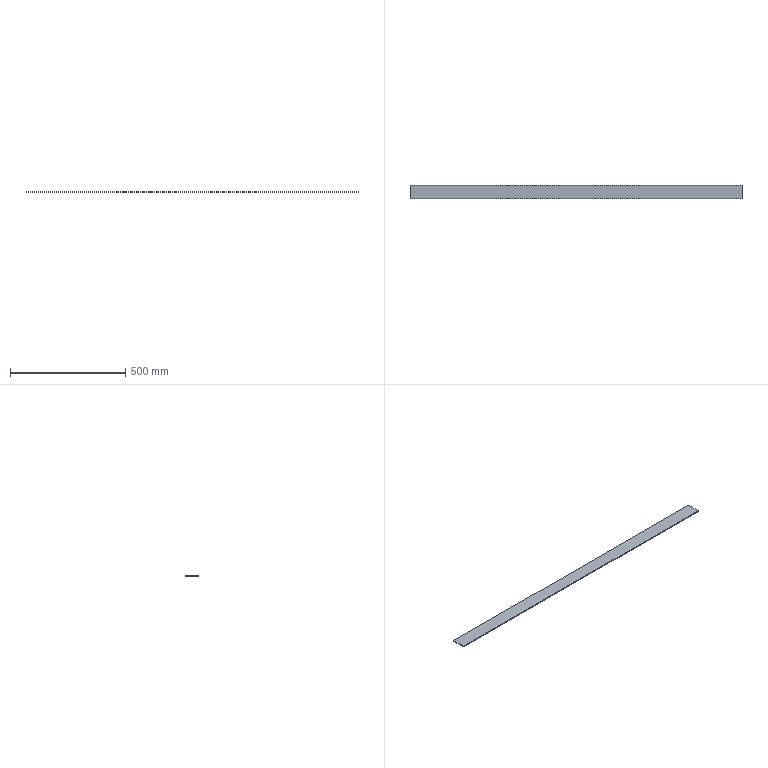Part | STEP file | 07-Rib plate | 1 solid | 6 faces | box 1440 x 60 x 4 mm | volume 345600 mm3 | plane 6
STEP:
#1=CARTESIAN_POINT('',(0.,0.,0.));
#2=DIRECTION('',(0.,0.,1.));
#3=DIRECTION('',(1.,0.,0.));
#4=AXIS2_PLACEMENT_3D('',#1,#2,#3);
#5=CARTESIAN_POINT('',(0.,0.,0.));
#6=VERTEX_POINT('',#5);
#7=CARTESIAN_POINT('',(0.,-60.,0.));
#8=VERTEX_POINT('',#7);
#9=CARTESIAN_POINT('',(0.,0.,0.));
#10=DIRECTION('',(0.,-1.,0.));
#11=VECTOR('',#10,1.);
#12=LINE('',#9,#11);
#13=CARTESIAN_POINT('',(0.,0.,4.));
#14=DIRECTION('',(1.,0.,0.));
#15=DIRECTION('',(0.,1.,0.));
#16=AXIS2_PLACEMENT_3D('',#13,#14,#15);
#17=PLANE('',#16);
#18=CARTESIAN_POINT('',(0.,-4.));
#19=DIRECTION('',(-1.,0.));
#20=VECTOR('',#19,1.);
#21=LINE('',#18,#20);
#22=(GEOMETRIC_REPRESENTATION_CONTEXT(2)PARAMETRIC_REPRESENTATION_CONTEXT()REPRESENTATION_CONTEXT('',''));
#23=DEFINITIONAL_REPRESENTATION('',(#21),#22);
#24=PCURVE('',#17,#23);
#25=CARTESIAN_POINT('',(0.,0.,0.));
#26=DIRECTION('',(0.,0.,1.));
#27=DIRECTION('',(1.,0.,0.));
#28=AXIS2_PLACEMENT_3D('',#25,#26,#27);
#29=PLANE('',#28);
#30=CARTESIAN_POINT('',(0.,0.));
#31=DIRECTION('',(0.,-1.));
#32=VECTOR('',#31,1.);
#33=LINE('',#30,#32);
#34=(GEOMETRIC_REPRESENTATION_CONTEXT(2)PARAMETRIC_REPRESENTATION_CONTEXT()REPRESENTATION_CONTEXT('',''));
#35=DEFINITIONAL_REPRESENTATION('',(#33),#34);
#36=PCURVE('',#29,#35);
#37=SURFACE_CURVE('',#12,(#24,#36),.PCURVE_S1.);
#38=EDGE_CURVE('',#6,#8,#37,.T.);
#39=ORIENTED_EDGE('',*,*,#38,.T.);
#40=CARTESIAN_POINT('',(0.,-60.,4.));
#41=VERTEX_POINT('',#40);
#42=CARTESIAN_POINT('',(0.,-60.,4.));
#43=DIRECTION('',(0.,0.,-1.));
#44=VECTOR('',#43,1.);
#45=LINE('',#42,#44);
#46=CARTESIAN_POINT('',(-60.,0.));
#47=DIRECTION('',(0.,-1.));
#48=VECTOR('',#47,1.);
#49=LINE('',#46,#48);
#50=(GEOMETRIC_REPRESENTATION_CONTEXT(2)PARAMETRIC_REPRESENTATION_CONTEXT()REPRESENTATION_CONTEXT('',''));
#51=DEFINITIONAL_REPRESENTATION('',(#49),#50);
#52=PCURVE('',#17,#51);
#53=CARTESIAN_POINT('',(0.,-60.,4.));
#54=DIRECTION('',(0.,1.,0.));
#55=DIRECTION('',(0.,0.,1.));
#56=AXIS2_PLACEMENT_3D('',#53,#54,#55);
#57=PLANE('',#56);
#58=CARTESIAN_POINT('',(0.,0.));
#59=DIRECTION('',(-1.,0.));
#60=VECTOR('',#59,1.);
#61=LINE('',#58,#60);
#62=(GEOMETRIC_REPRESENTATION_CONTEXT(2)PARAMETRIC_REPRESENTATION_CONTEXT()REPRESENTATION_CONTEXT('',''));
#63=DEFINITIONAL_REPRESENTATION('',(#61),#62);
#64=PCURVE('',#57,#63);
#65=SURFACE_CURVE('',#45,(#52,#64),.PCURVE_S1.);
#66=EDGE_CURVE('',#41,#8,#65,.T.);
#67=ORIENTED_EDGE('',*,*,#66,.F.);
#68=CARTESIAN_POINT('',(0.,0.,4.));
#69=VERTEX_POINT('',#68);
#70=CARTESIAN_POINT('',(0.,0.,4.));
#71=DIRECTION('',(0.,-1.,0.));
#72=VECTOR('',#71,1.);
#73=LINE('',#70,#72);
#74=CARTESIAN_POINT('',(0.,0.));
#75=DIRECTION('',(-1.,0.));
#76=VECTOR('',#75,1.);
#77=LINE('',#74,#76);
#78=(GEOMETRIC_REPRESENTATION_CONTEXT(2)PARAMETRIC_REPRESENTATION_CONTEXT()REPRESENTATION_CONTEXT('',''));
#79=DEFINITIONAL_REPRESENTATION('',(#77),#78);
#80=PCURVE('',#17,#79);
#81=CARTESIAN_POINT('',(0.,0.,4.));
#82=DIRECTION('',(0.,0.,1.));
#83=DIRECTION('',(1.,0.,0.));
#84=AXIS2_PLACEMENT_3D('',#81,#82,#83);
#85=PLANE('',#84);
#86=CARTESIAN_POINT('',(0.,0.));
#87=DIRECTION('',(0.,-1.));
#88=VECTOR('',#87,1.);
#89=LINE('',#86,#88);
#90=(GEOMETRIC_REPRESENTATION_CONTEXT(2)PARAMETRIC_REPRESENTATION_CONTEXT()REPRESENTATION_CONTEXT('',''));
#91=DEFINITIONAL_REPRESENTATION('',(#89),#90);
#92=PCURVE('',#85,#91);
#93=SURFACE_CURVE('',#73,(#80,#92),.PCURVE_S1.);
#94=EDGE_CURVE('',#69,#41,#93,.T.);
#95=ORIENTED_EDGE('',*,*,#94,.F.);
#96=CARTESIAN_POINT('',(0.,0.,4.));
#97=DIRECTION('',(0.,0.,-1.));
#98=VECTOR('',#97,1.);
#99=LINE('',#96,#98);
#100=CARTESIAN_POINT('',(0.,0.));
#101=DIRECTION('',(0.,-1.));
#102=VECTOR('',#101,1.);
#103=LINE('',#100,#102);
#104=(GEOMETRIC_REPRESENTATION_CONTEXT(2)PARAMETRIC_REPRESENTATION_CONTEXT()REPRESENTATION_CONTEXT('',''));
#105=DEFINITIONAL_REPRESENTATION('',(#103),#104);
#106=PCURVE('',#17,#105);
#107=CARTESIAN_POINT('',(0.,0.,4.));
#108=DIRECTION('',(0.,-1.,0.));
#109=DIRECTION('',(0.,0.,-1.));
#110=AXIS2_PLACEMENT_3D('',#107,#108,#109);
#111=PLANE('',#110);
#112=CARTESIAN_POINT('',(0.,0.));
#113=DIRECTION('',(1.,0.));
#114=VECTOR('',#113,1.);
#115=LINE('',#112,#114);
#116=(GEOMETRIC_REPRESENTATION_CONTEXT(2)PARAMETRIC_REPRESENTATION_CONTEXT()REPRESENTATION_CONTEXT('',''));
#117=DEFINITIONAL_REPRESENTATION('',(#115),#116);
#118=PCURVE('',#111,#117);
#119=SURFACE_CURVE('',#99,(#106,#118),.PCURVE_S1.);
#120=EDGE_CURVE('',#69,#6,#119,.T.);
#121=ORIENTED_EDGE('',*,*,#120,.T.);
#122=EDGE_LOOP('',(#39,#67,#95,#121));
#123=FACE_BOUND('',#122,.T.);
#124=ADVANCED_FACE('',(#123),#17,.F.);
#125=CARTESIAN_POINT('',(1440.,-60.,0.));
#126=VERTEX_POINT('',#125);
#127=CARTESIAN_POINT('',(0.,-60.,0.));
#128=DIRECTION('',(1.,0.,0.));
#129=VECTOR('',#128,1.);
#130=LINE('',#127,#129);
#131=CARTESIAN_POINT('',(-4.,0.));
#132=DIRECTION('',(0.,1.));
#133=VECTOR('',#132,1.);
#134=LINE('',#131,#133);
#135=(GEOMETRIC_REPRESENTATION_CONTEXT(2)PARAMETRIC_REPRESENTATION_CONTEXT()REPRESENTATION_CONTEXT('',''));
#136=DEFINITIONAL_REPRESENTATION('',(#134),#135);
#137=PCURVE('',#57,#136);
#138=CARTESIAN_POINT('',(0.,-60.));
#139=DIRECTION('',(1.,0.));
#140=VECTOR('',#139,1.);
#141=LINE('',#138,#140);
#142=(GEOMETRIC_REPRESENTATION_CONTEXT(2)PARAMETRIC_REPRESENTATION_CONTEXT()REPRESENTATION_CONTEXT('',''));
#143=DEFINITIONAL_REPRESENTATION('',(#141),#142);
#144=PCURVE('',#29,#143);
#145=SURFACE_CURVE('',#130,(#137,#144),.PCURVE_S1.);
#146=EDGE_CURVE('',#8,#126,#145,.T.);
#147=ORIENTED_EDGE('',*,*,#146,.T.);
#148=CARTESIAN_POINT('',(1440.,-60.,4.));
#149=VERTEX_POINT('',#148);
#150=CARTESIAN_POINT('',(1440.,-60.,4.));
#151=DIRECTION('',(0.,0.,-1.));
#152=VECTOR('',#151,1.);
#153=LINE('',#150,#152);
#154=CARTESIAN_POINT('',(0.,1440.));
#155=DIRECTION('',(-1.,0.));
#156=VECTOR('',#155,1.);
#157=LINE('',#154,#156);
#158=(GEOMETRIC_REPRESENTATION_CONTEXT(2)PARAMETRIC_REPRESENTATION_CONTEXT()REPRESENTATION_CONTEXT('',''));
#159=DEFINITIONAL_REPRESENTATION('',(#157),#158);
#160=PCURVE('',#57,#159);
#161=CARTESIAN_POINT('',(1440.,0.,4.));
#162=DIRECTION('',(-1.,0.,0.));
#163=DIRECTION('',(0.,0.,1.));
#164=AXIS2_PLACEMENT_3D('',#161,#162,#163);
#165=PLANE('',#164);
#166=CARTESIAN_POINT('',(0.,-60.));
#167=DIRECTION('',(-1.,0.));
#168=VECTOR('',#167,1.);
#169=LINE('',#166,#168);
#170=(GEOMETRIC_REPRESENTATION_CONTEXT(2)PARAMETRIC_REPRESENTATION_CONTEXT()REPRESENTATION_CONTEXT('',''));
#171=DEFINITIONAL_REPRESENTATION('',(#169),#170);
#172=PCURVE('',#165,#171);
#173=SURFACE_CURVE('',#153,(#160,#172),.PCURVE_S1.);
#174=EDGE_CURVE('',#149,#126,#173,.T.);
#175=ORIENTED_EDGE('',*,*,#174,.F.);
#176=CARTESIAN_POINT('',(0.,-60.,4.));
#177=DIRECTION('',(1.,0.,0.));
#178=VECTOR('',#177,1.);
#179=LINE('',#176,#178);
#180=CARTESIAN_POINT('',(0.,0.));
#181=DIRECTION('',(0.,1.));
#182=VECTOR('',#181,1.);
#183=LINE('',#180,#182);
#184=(GEOMETRIC_REPRESENTATION_CONTEXT(2)PARAMETRIC_REPRESENTATION_CONTEXT()REPRESENTATION_CONTEXT('',''));
#185=DEFINITIONAL_REPRESENTATION('',(#183),#184);
#186=PCURVE('',#57,#185);
#187=CARTESIAN_POINT('',(0.,-60.));
#188=DIRECTION('',(1.,0.));
#189=VECTOR('',#188,1.);
#190=LINE('',#187,#189);
#191=(GEOMETRIC_REPRESENTATION_CONTEXT(2)PARAMETRIC_REPRESENTATION_CONTEXT()REPRESENTATION_CONTEXT('',''));
#192=DEFINITIONAL_REPRESENTATION('',(#190),#191);
#193=PCURVE('',#85,#192);
#194=SURFACE_CURVE('',#179,(#186,#193),.PCURVE_S1.);
#195=EDGE_CURVE('',#41,#149,#194,.T.);
#196=ORIENTED_EDGE('',*,*,#195,.F.);
#197=ORIENTED_EDGE('',*,*,#66,.T.);
#198=EDGE_LOOP('',(#147,#175,#196,#197));
#199=FACE_BOUND('',#198,.T.);
#200=ADVANCED_FACE('',(#199),#57,.F.);
#201=CARTESIAN_POINT('',(1440.,0.,0.));
#202=VERTEX_POINT('',#201);
#203=CARTESIAN_POINT('',(1440.,0.,0.));
#204=DIRECTION('',(0.,1.,0.));
#205=VECTOR('',#204,1.);
#206=LINE('',#203,#205);
#207=CARTESIAN_POINT('',(-4.,0.));
#208=DIRECTION('',(0.,1.));
#209=VECTOR('',#208,1.);
#210=LINE('',#207,#209);
#211=(GEOMETRIC_REPRESENTATION_CONTEXT(2)PARAMETRIC_REPRESENTATION_CONTEXT()REPRESENTATION_CONTEXT('',''));
#212=DEFINITIONAL_REPRESENTATION('',(#210),#211);
#213=PCURVE('',#165,#212);
#214=CARTESIAN_POINT('',(1440.,0.));
#215=DIRECTION('',(0.,1.));
#216=VECTOR('',#215,1.);
#217=LINE('',#214,#216);
#218=(GEOMETRIC_REPRESENTATION_CONTEXT(2)PARAMETRIC_REPRESENTATION_CONTEXT()REPRESENTATION_CONTEXT('',''));
#219=DEFINITIONAL_REPRESENTATION('',(#217),#218);
#220=PCURVE('',#29,#219);
#221=SURFACE_CURVE('',#206,(#213,#220),.PCURVE_S1.);
#222=EDGE_CURVE('',#126,#202,#221,.T.);
#223=ORIENTED_EDGE('',*,*,#222,.T.);
#224=CARTESIAN_POINT('',(1440.,0.,4.));
#225=VERTEX_POINT('',#224);
#226=CARTESIAN_POINT('',(1440.,0.,4.));
#227=DIRECTION('',(0.,0.,-1.));
#228=VECTOR('',#227,1.);
#229=LINE('',#226,#228);
#230=CARTESIAN_POINT('',(0.,0.));
#231=DIRECTION('',(-1.,0.));
#232=VECTOR('',#231,1.);
#233=LINE('',#230,#232);
#234=(GEOMETRIC_REPRESENTATION_CONTEXT(2)PARAMETRIC_REPRESENTATION_CONTEXT()REPRESENTATION_CONTEXT('',''));
#235=DEFINITIONAL_REPRESENTATION('',(#233),#234);
#236=PCURVE('',#165,#235);
#237=CARTESIAN_POINT('',(0.,1440.));
#238=DIRECTION('',(1.,0.));
#239=VECTOR('',#238,1.);
#240=LINE('',#237,#239);
#241=(GEOMETRIC_REPRESENTATION_CONTEXT(2)PARAMETRIC_REPRESENTATION_CONTEXT()REPRESENTATION_CONTEXT('',''));
#242=DEFINITIONAL_REPRESENTATION('',(#240),#241);
#243=PCURVE('',#111,#242);
#244=SURFACE_CURVE('',#229,(#236,#243),.PCURVE_S1.);
#245=EDGE_CURVE('',#225,#202,#244,.T.);
#246=ORIENTED_EDGE('',*,*,#245,.F.);
#247=CARTESIAN_POINT('',(1440.,0.,4.));
#248=DIRECTION('',(0.,1.,0.));
#249=VECTOR('',#248,1.);
#250=LINE('',#247,#249);
#251=CARTESIAN_POINT('',(0.,0.));
#252=DIRECTION('',(0.,1.));
#253=VECTOR('',#252,1.);
#254=LINE('',#251,#253);
#255=(GEOMETRIC_REPRESENTATION_CONTEXT(2)PARAMETRIC_REPRESENTATION_CONTEXT()REPRESENTATION_CONTEXT('',''));
#256=DEFINITIONAL_REPRESENTATION('',(#254),#255);
#257=PCURVE('',#165,#256);
#258=CARTESIAN_POINT('',(1440.,0.));
#259=DIRECTION('',(0.,1.));
#260=VECTOR('',#259,1.);
#261=LINE('',#258,#260);
#262=(GEOMETRIC_REPRESENTATION_CONTEXT(2)PARAMETRIC_REPRESENTATION_CONTEXT()REPRESENTATION_CONTEXT('',''));
#263=DEFINITIONAL_REPRESENTATION('',(#261),#262);
#264=PCURVE('',#85,#263);
#265=SURFACE_CURVE('',#250,(#257,#264),.PCURVE_S1.);
#266=EDGE_CURVE('',#149,#225,#265,.T.);
#267=ORIENTED_EDGE('',*,*,#266,.F.);
#268=ORIENTED_EDGE('',*,*,#174,.T.);
#269=EDGE_LOOP('',(#223,#246,#267,#268));
#270=FACE_BOUND('',#269,.T.);
#271=ADVANCED_FACE('',(#270),#165,.F.);
#272=CARTESIAN_POINT('',(0.,0.,0.));
#273=DIRECTION('',(-1.,0.,0.));
#274=VECTOR('',#273,1.);
#275=LINE('',#272,#274);
#276=CARTESIAN_POINT('',(4.,0.));
#277=DIRECTION('',(0.,-1.));
#278=VECTOR('',#277,1.);
#279=LINE('',#276,#278);
#280=(GEOMETRIC_REPRESENTATION_CONTEXT(2)PARAMETRIC_REPRESENTATION_CONTEXT()REPRESENTATION_CONTEXT('',''));
#281=DEFINITIONAL_REPRESENTATION('',(#279),#280);
#282=PCURVE('',#111,#281);
#283=CARTESIAN_POINT('',(0.,0.));
#284=DIRECTION('',(-1.,0.));
#285=VECTOR('',#284,1.);
#286=LINE('',#283,#285);
#287=(GEOMETRIC_REPRESENTATION_CONTEXT(2)PARAMETRIC_REPRESENTATION_CONTEXT()REPRESENTATION_CONTEXT('',''));
#288=DEFINITIONAL_REPRESENTATION('',(#286),#287);
#289=PCURVE('',#29,#288);
#290=SURFACE_CURVE('',#275,(#282,#289),.PCURVE_S1.);
#291=EDGE_CURVE('',#202,#6,#290,.T.);
#292=ORIENTED_EDGE('',*,*,#291,.T.);
#293=ORIENTED_EDGE('',*,*,#120,.F.);
#294=CARTESIAN_POINT('',(0.,0.,4.));
#295=DIRECTION('',(-1.,0.,0.));
#296=VECTOR('',#295,1.);
#297=LINE('',#294,#296);
#298=CARTESIAN_POINT('',(0.,0.));
#299=DIRECTION('',(0.,-1.));
#300=VECTOR('',#299,1.);
#301=LINE('',#298,#300);
#302=(GEOMETRIC_REPRESENTATION_CONTEXT(2)PARAMETRIC_REPRESENTATION_CONTEXT()REPRESENTATION_CONTEXT('',''));
#303=DEFINITIONAL_REPRESENTATION('',(#301),#302);
#304=PCURVE('',#111,#303);
#305=CARTESIAN_POINT('',(0.,0.));
#306=DIRECTION('',(-1.,0.));
#307=VECTOR('',#306,1.);
#308=LINE('',#305,#307);
#309=(GEOMETRIC_REPRESENTATION_CONTEXT(2)PARAMETRIC_REPRESENTATION_CONTEXT()REPRESENTATION_CONTEXT('',''));
#310=DEFINITIONAL_REPRESENTATION('',(#308),#309);
#311=PCURVE('',#85,#310);
#312=SURFACE_CURVE('',#297,(#304,#311),.PCURVE_S1.);
#313=EDGE_CURVE('',#225,#69,#312,.T.);
#314=ORIENTED_EDGE('',*,*,#313,.F.);
#315=ORIENTED_EDGE('',*,*,#245,.T.);
#316=EDGE_LOOP('',(#292,#293,#314,#315));
#317=FACE_BOUND('',#316,.T.);
#318=ADVANCED_FACE('',(#317),#111,.F.);
#319=ORIENTED_EDGE('',*,*,#94,.T.);
#320=ORIENTED_EDGE('',*,*,#195,.T.);
#321=ORIENTED_EDGE('',*,*,#266,.T.);
#322=ORIENTED_EDGE('',*,*,#313,.T.);
#323=EDGE_LOOP('',(#319,#320,#321,#322));
#324=FACE_BOUND('',#323,.T.);
#325=ADVANCED_FACE('',(#324),#85,.T.);
#326=ORIENTED_EDGE('',*,*,#38,.F.);
#327=ORIENTED_EDGE('',*,*,#291,.F.);
#328=ORIENTED_EDGE('',*,*,#222,.F.);
#329=ORIENTED_EDGE('',*,*,#146,.F.);
#330=EDGE_LOOP('',(#326,#327,#328,#329));
#331=FACE_BOUND('',#330,.T.);
#332=ADVANCED_FACE('',(#331),#29,.F.);
#333=CLOSED_SHELL('',(#124,#200,#271,#318,#325,#332));
#334=MANIFOLD_SOLID_BREP('',#333);
#335=(LENGTH_UNIT()NAMED_UNIT(*)SI_UNIT(.MILLI.,.METRE.));
#336=UNCERTAINTY_MEASURE_WITH_UNIT(LENGTH_MEASURE(0.0000001),#335,'','');
#337=(NAMED_UNIT(*)PLANE_ANGLE_UNIT()SI_UNIT($,.RADIAN.));
#338=(NAMED_UNIT(*)SI_UNIT($,.STERADIAN.)SOLID_ANGLE_UNIT());
#339=(GEOMETRIC_REPRESENTATION_CONTEXT(3)GLOBAL_UNCERTAINTY_ASSIGNED_CONTEXT((#336))GLOBAL_UNIT_ASSIGNED_CONTEXT((#335,#337,#338))REPRESENTATION_CONTEXT('',''));
#340=ADVANCED_BREP_SHAPE_REPRESENTATION('',(#4,#334),#339);